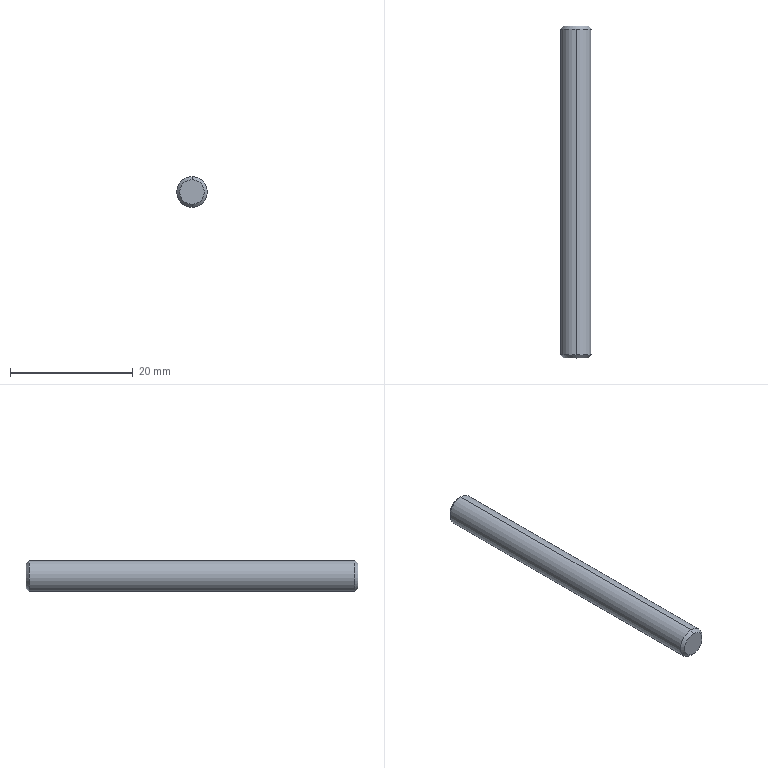Part | STEP file | SecondRearHHPMGS6pin_Default | 1 solid | 8 faces | box 5 x 54 x 5 mm | volume 1057 mm3 | cone 4 | cylinder 2 | plane 2 | commonest cylinder face diameters 5 x2
STEP:
#1=CARTESIAN_POINT('',(0.,0.,0.));
#2=DIRECTION('',(0.,0.,1.));
#3=DIRECTION('',(1.,0.,0.));
#4=AXIS2_PLACEMENT_3D('',#1,#2,#3);
#5=CARTESIAN_POINT('',(0.,-27.,2.));
#6=VERTEX_POINT('',#5);
#7=CARTESIAN_POINT('',(0.,-27.,-2.));
#8=VERTEX_POINT('',#7);
#9=CARTESIAN_POINT('',(0.,-27.,0.));
#10=DIRECTION('',(0.,1.,0.));
#11=DIRECTION('',(0.,0.,1.));
#12=AXIS2_PLACEMENT_3D('',#9,#10,#11);
#13=CIRCLE('',#12,2.);
#14=CARTESIAN_POINT('',(0.,-27.,0.));
#15=DIRECTION('',(0.,1.,0.));
#16=DIRECTION('',(0.,0.,1.));
#17=AXIS2_PLACEMENT_3D('',#14,#15,#16);
#18=CONICAL_SURFACE('',#17,2.,0.7854);
#19=CARTESIAN_POINT('',(0.,0.));
#20=DIRECTION('',(1.,0.));
#21=VECTOR('',#20,1.);
#22=LINE('',#19,#21);
#23=(GEOMETRIC_REPRESENTATION_CONTEXT(2)PARAMETRIC_REPRESENTATION_CONTEXT()REPRESENTATION_CONTEXT('',''));
#24=DEFINITIONAL_REPRESENTATION('',(#22),#23);
#25=PCURVE('',#18,#24);
#26=CARTESIAN_POINT('',(2.,-27.,0.));
#27=DIRECTION('',(0.,1.,0.));
#28=DIRECTION('',(0.,0.,1.));
#29=AXIS2_PLACEMENT_3D('',#26,#27,#28);
#30=PLANE('',#29);
#31=CARTESIAN_POINT('',(0.,-2.));
#32=DIRECTION('',(1.,0.));
#33=AXIS2_PLACEMENT_2D('',#31,#32);
#34=CIRCLE('',#33,2.);
#35=(GEOMETRIC_REPRESENTATION_CONTEXT(2)PARAMETRIC_REPRESENTATION_CONTEXT()REPRESENTATION_CONTEXT('',''));
#36=DEFINITIONAL_REPRESENTATION('',(#34),#35);
#37=PCURVE('',#30,#36);
#38=SURFACE_CURVE('',#13,(#25,#37),.PCURVE_S1.);
#39=EDGE_CURVE('',#6,#8,#38,.T.);
#40=ORIENTED_EDGE('',*,*,#39,.T.);
#41=CARTESIAN_POINT('',(0.,-26.5,-2.5));
#42=VERTEX_POINT('',#41);
#43=CARTESIAN_POINT('',(0.,-27.,-2.));
#44=DIRECTION('',(0.,0.7071,-0.7071));
#45=VECTOR('',#44,1.);
#46=LINE('',#43,#45);
#47=CARTESIAN_POINT('',(3.142,0.));
#48=DIRECTION('',(0.,1.));
#49=VECTOR('',#48,1.);
#50=LINE('',#47,#49);
#51=(GEOMETRIC_REPRESENTATION_CONTEXT(2)PARAMETRIC_REPRESENTATION_CONTEXT()REPRESENTATION_CONTEXT('',''));
#52=DEFINITIONAL_REPRESENTATION('',(#50),#51);
#53=PCURVE('',#18,#52);
#54=CARTESIAN_POINT('',(0.,-27.,0.));
#55=DIRECTION('',(0.,1.,0.));
#56=DIRECTION('',(0.,0.,1.));
#57=AXIS2_PLACEMENT_3D('',#54,#55,#56);
#58=CONICAL_SURFACE('',#57,2.,0.7854);
#59=CARTESIAN_POINT('',(3.142,0.));
#60=DIRECTION('',(0.,1.));
#61=VECTOR('',#60,1.);
#62=LINE('',#59,#61);
#63=(GEOMETRIC_REPRESENTATION_CONTEXT(2)PARAMETRIC_REPRESENTATION_CONTEXT()REPRESENTATION_CONTEXT('',''));
#64=DEFINITIONAL_REPRESENTATION('',(#62),#63);
#65=PCURVE('',#58,#64);
#66=SURFACE_CURVE('',#46,(#53,#65),.PCURVE_S1.);
#67=EDGE_CURVE('',#8,#42,#66,.T.);
#68=ORIENTED_EDGE('',*,*,#67,.T.);
#69=CARTESIAN_POINT('',(0.,-26.5,2.5));
#70=VERTEX_POINT('',#69);
#71=CARTESIAN_POINT('',(0.,-26.5,0.));
#72=DIRECTION('',(0.,1.,0.));
#73=DIRECTION('',(0.,0.,1.));
#74=AXIS2_PLACEMENT_3D('',#71,#72,#73);
#75=CIRCLE('',#74,2.5);
#76=CARTESIAN_POINT('',(0.,0.5));
#77=DIRECTION('',(1.,0.));
#78=VECTOR('',#77,1.);
#79=LINE('',#76,#78);
#80=(GEOMETRIC_REPRESENTATION_CONTEXT(2)PARAMETRIC_REPRESENTATION_CONTEXT()REPRESENTATION_CONTEXT('',''));
#81=DEFINITIONAL_REPRESENTATION('',(#79),#80);
#82=PCURVE('',#18,#81);
#83=CARTESIAN_POINT('',(0.,-27.,0.));
#84=DIRECTION('',(0.,1.,0.));
#85=DIRECTION('',(0.,0.,1.));
#86=AXIS2_PLACEMENT_3D('',#83,#84,#85);
#87=CYLINDRICAL_SURFACE('',#86,2.5);
#88=CARTESIAN_POINT('',(0.,0.5));
#89=DIRECTION('',(1.,0.));
#90=VECTOR('',#89,1.);
#91=LINE('',#88,#90);
#92=(GEOMETRIC_REPRESENTATION_CONTEXT(2)PARAMETRIC_REPRESENTATION_CONTEXT()REPRESENTATION_CONTEXT('',''));
#93=DEFINITIONAL_REPRESENTATION('',(#91),#92);
#94=PCURVE('',#87,#93);
#95=SURFACE_CURVE('',#75,(#82,#94),.PCURVE_S1.);
#96=EDGE_CURVE('',#70,#42,#95,.T.);
#97=ORIENTED_EDGE('',*,*,#96,.F.);
#98=CARTESIAN_POINT('',(0.,-27.,2.));
#99=DIRECTION('',(0.,0.7071,0.7071));
#100=VECTOR('',#99,1.);
#101=LINE('',#98,#100);
#102=CARTESIAN_POINT('',(0.,0.));
#103=DIRECTION('',(0.,1.));
#104=VECTOR('',#103,1.);
#105=LINE('',#102,#104);
#106=(GEOMETRIC_REPRESENTATION_CONTEXT(2)PARAMETRIC_REPRESENTATION_CONTEXT()REPRESENTATION_CONTEXT('',''));
#107=DEFINITIONAL_REPRESENTATION('',(#105),#106);
#108=PCURVE('',#18,#107);
#109=CARTESIAN_POINT('',(6.283,0.));
#110=DIRECTION('',(0.,1.));
#111=VECTOR('',#110,1.);
#112=LINE('',#109,#111);
#113=(GEOMETRIC_REPRESENTATION_CONTEXT(2)PARAMETRIC_REPRESENTATION_CONTEXT()REPRESENTATION_CONTEXT('',''));
#114=DEFINITIONAL_REPRESENTATION('',(#112),#113);
#115=PCURVE('',#58,#114);
#116=SURFACE_CURVE('',#101,(#108,#115),.PCURVE_S1.);
#117=EDGE_CURVE('',#6,#70,#116,.T.);
#118=ORIENTED_EDGE('',*,*,#117,.F.);
#119=EDGE_LOOP('',(#40,#68,#97,#118));
#120=FACE_BOUND('',#119,.T.);
#121=ADVANCED_FACE('',(#120),#18,.T.);
#122=ORIENTED_EDGE('',*,*,#96,.T.);
#123=CARTESIAN_POINT('',(0.,26.5,-2.5));
#124=VERTEX_POINT('',#123);
#125=CARTESIAN_POINT('',(0.,-27.,-2.5));
#126=DIRECTION('',(0.,1.,0.));
#127=VECTOR('',#126,1.);
#128=LINE('',#125,#127);
#129=CARTESIAN_POINT('',(3.142,0.));
#130=DIRECTION('',(0.,1.));
#131=VECTOR('',#130,1.);
#132=LINE('',#129,#131);
#133=(GEOMETRIC_REPRESENTATION_CONTEXT(2)PARAMETRIC_REPRESENTATION_CONTEXT()REPRESENTATION_CONTEXT('',''));
#134=DEFINITIONAL_REPRESENTATION('',(#132),#133);
#135=PCURVE('',#87,#134);
#136=CARTESIAN_POINT('',(0.,-27.,0.));
#137=DIRECTION('',(0.,1.,0.));
#138=DIRECTION('',(0.,0.,1.));
#139=AXIS2_PLACEMENT_3D('',#136,#137,#138);
#140=CYLINDRICAL_SURFACE('',#139,2.5);
#141=CARTESIAN_POINT('',(3.142,0.));
#142=DIRECTION('',(0.,1.));
#143=VECTOR('',#142,1.);
#144=LINE('',#141,#143);
#145=(GEOMETRIC_REPRESENTATION_CONTEXT(2)PARAMETRIC_REPRESENTATION_CONTEXT()REPRESENTATION_CONTEXT('',''));
#146=DEFINITIONAL_REPRESENTATION('',(#144),#145);
#147=PCURVE('',#140,#146);
#148=SURFACE_CURVE('',#128,(#135,#147),.PCURVE_S1.);
#149=EDGE_CURVE('',#42,#124,#148,.T.);
#150=ORIENTED_EDGE('',*,*,#149,.T.);
#151=CARTESIAN_POINT('',(0.,26.5,2.5));
#152=VERTEX_POINT('',#151);
#153=CARTESIAN_POINT('',(0.,26.5,0.));
#154=DIRECTION('',(0.,1.,0.));
#155=DIRECTION('',(0.,0.,1.));
#156=AXIS2_PLACEMENT_3D('',#153,#154,#155);
#157=CIRCLE('',#156,2.5);
#158=CARTESIAN_POINT('',(0.,53.5));
#159=DIRECTION('',(1.,0.));
#160=VECTOR('',#159,1.);
#161=LINE('',#158,#160);
#162=(GEOMETRIC_REPRESENTATION_CONTEXT(2)PARAMETRIC_REPRESENTATION_CONTEXT()REPRESENTATION_CONTEXT('',''));
#163=DEFINITIONAL_REPRESENTATION('',(#161),#162);
#164=PCURVE('',#87,#163);
#165=CARTESIAN_POINT('',(0.,26.5,0.));
#166=DIRECTION('',(0.,-1.,0.));
#167=DIRECTION('',(0.,0.,-1.));
#168=AXIS2_PLACEMENT_3D('',#165,#166,#167);
#169=CONICAL_SURFACE('',#168,2.5,0.7854);
#170=CARTESIAN_POINT('',(3.142,0.));
#171=DIRECTION('',(-1.,0.));
#172=VECTOR('',#171,1.);
#173=LINE('',#170,#172);
#174=(GEOMETRIC_REPRESENTATION_CONTEXT(2)PARAMETRIC_REPRESENTATION_CONTEXT()REPRESENTATION_CONTEXT('',''));
#175=DEFINITIONAL_REPRESENTATION('',(#173),#174);
#176=PCURVE('',#169,#175);
#177=SURFACE_CURVE('',#157,(#164,#176),.PCURVE_S1.);
#178=EDGE_CURVE('',#152,#124,#177,.T.);
#179=ORIENTED_EDGE('',*,*,#178,.F.);
#180=CARTESIAN_POINT('',(0.,-27.,2.5));
#181=DIRECTION('',(0.,1.,0.));
#182=VECTOR('',#181,1.);
#183=LINE('',#180,#182);
#184=CARTESIAN_POINT('',(0.,0.));
#185=DIRECTION('',(0.,1.));
#186=VECTOR('',#185,1.);
#187=LINE('',#184,#186);
#188=(GEOMETRIC_REPRESENTATION_CONTEXT(2)PARAMETRIC_REPRESENTATION_CONTEXT()REPRESENTATION_CONTEXT('',''));
#189=DEFINITIONAL_REPRESENTATION('',(#187),#188);
#190=PCURVE('',#87,#189);
#191=CARTESIAN_POINT('',(6.283,0.));
#192=DIRECTION('',(0.,1.));
#193=VECTOR('',#192,1.);
#194=LINE('',#191,#193);
#195=(GEOMETRIC_REPRESENTATION_CONTEXT(2)PARAMETRIC_REPRESENTATION_CONTEXT()REPRESENTATION_CONTEXT('',''));
#196=DEFINITIONAL_REPRESENTATION('',(#194),#195);
#197=PCURVE('',#140,#196);
#198=SURFACE_CURVE('',#183,(#190,#197),.PCURVE_S1.);
#199=EDGE_CURVE('',#70,#152,#198,.T.);
#200=ORIENTED_EDGE('',*,*,#199,.F.);
#201=EDGE_LOOP('',(#122,#150,#179,#200));
#202=FACE_BOUND('',#201,.T.);
#203=ADVANCED_FACE('',(#202),#87,.T.);
#204=CARTESIAN_POINT('',(0.,27.,2.));
#205=VERTEX_POINT('',#204);
#206=CARTESIAN_POINT('',(0.,27.,-2.));
#207=VERTEX_POINT('',#206);
#208=CARTESIAN_POINT('',(0.,27.,0.));
#209=DIRECTION('',(0.,1.,0.));
#210=DIRECTION('',(0.,0.,1.));
#211=AXIS2_PLACEMENT_3D('',#208,#209,#210);
#212=CIRCLE('',#211,2.);
#213=CARTESIAN_POINT('',(3.142,-0.5));
#214=DIRECTION('',(-1.,0.));
#215=VECTOR('',#214,1.);
#216=LINE('',#213,#215);
#217=(GEOMETRIC_REPRESENTATION_CONTEXT(2)PARAMETRIC_REPRESENTATION_CONTEXT()REPRESENTATION_CONTEXT('',''));
#218=DEFINITIONAL_REPRESENTATION('',(#216),#217);
#219=PCURVE('',#169,#218);
#220=CARTESIAN_POINT('',(0.,27.,0.));
#221=DIRECTION('',(0.,-1.,0.));
#222=DIRECTION('',(0.,0.,-1.));
#223=AXIS2_PLACEMENT_3D('',#220,#221,#222);
#224=PLANE('',#223);
#225=CARTESIAN_POINT('',(-2.,0.));
#226=CARTESIAN_POINT('',(-2.,3.464));
#227=CARTESIAN_POINT('',(1.,1.732));
#228=CARTESIAN_POINT('',(4.,0.));
#229=CARTESIAN_POINT('',(1.,-1.732));
#230=CARTESIAN_POINT('',(-2.,-3.464));
#231=CARTESIAN_POINT('',(-2.,0.));
#232=(BOUNDED_CURVE()B_SPLINE_CURVE(2,(#225,#226,#227,#228,#229,#230,#231),.UNSPECIFIED.,.T.,.F.)B_SPLINE_CURVE_WITH_KNOTS((1,2,2,2,2,1),(-2.094,0.,2.094,4.189,6.283,8.378),.UNSPECIFIED.)CURVE()GEOMETRIC_REPRESENTATION_ITEM()RATIONAL_B_SPLINE_CURVE((1.,0.5,1.,0.5,1.,0.5,1.))REPRESENTATION_ITEM(''));
#233=(GEOMETRIC_REPRESENTATION_CONTEXT(2)PARAMETRIC_REPRESENTATION_CONTEXT()REPRESENTATION_CONTEXT('',''));
#234=DEFINITIONAL_REPRESENTATION('',(#232),#233);
#235=PCURVE('',#224,#234);
#236=SURFACE_CURVE('',#212,(#219,#235),.PCURVE_S1.);
#237=EDGE_CURVE('',#205,#207,#236,.T.);
#238=ORIENTED_EDGE('',*,*,#237,.F.);
#239=CARTESIAN_POINT('',(0.,26.5,2.5));
#240=DIRECTION('',(0.,-0.7071,0.7071));
#241=VECTOR('',#240,1.);
#242=LINE('',#239,#241);
#243=CARTESIAN_POINT('',(3.142,0.));
#244=DIRECTION('',(0.,1.));
#245=VECTOR('',#244,1.);
#246=LINE('',#243,#245);
#247=(GEOMETRIC_REPRESENTATION_CONTEXT(2)PARAMETRIC_REPRESENTATION_CONTEXT()REPRESENTATION_CONTEXT('',''));
#248=DEFINITIONAL_REPRESENTATION('',(#246),#247);
#249=PCURVE('',#169,#248);
#250=CARTESIAN_POINT('',(0.,26.5,0.));
#251=DIRECTION('',(0.,-1.,0.));
#252=DIRECTION('',(0.,0.,-1.));
#253=AXIS2_PLACEMENT_3D('',#250,#251,#252);
#254=CONICAL_SURFACE('',#253,2.5,0.7854);
#255=CARTESIAN_POINT('',(3.142,0.));
#256=DIRECTION('',(0.,1.));
#257=VECTOR('',#256,1.);
#258=LINE('',#255,#257);
#259=(GEOMETRIC_REPRESENTATION_CONTEXT(2)PARAMETRIC_REPRESENTATION_CONTEXT()REPRESENTATION_CONTEXT('',''));
#260=DEFINITIONAL_REPRESENTATION('',(#258),#259);
#261=PCURVE('',#254,#260);
#262=SURFACE_CURVE('',#242,(#249,#261),.PCURVE_S1.);
#263=EDGE_CURVE('',#205,#152,#262,.T.);
#264=ORIENTED_EDGE('',*,*,#263,.T.);
#265=ORIENTED_EDGE('',*,*,#178,.T.);
#266=CARTESIAN_POINT('',(0.,26.5,-2.5));
#267=DIRECTION('',(0.,-0.7071,-0.7071));
#268=VECTOR('',#267,1.);
#269=LINE('',#266,#268);
#270=CARTESIAN_POINT('',(0.,0.));
#271=DIRECTION('',(0.,1.));
#272=VECTOR('',#271,1.);
#273=LINE('',#270,#272);
#274=(GEOMETRIC_REPRESENTATION_CONTEXT(2)PARAMETRIC_REPRESENTATION_CONTEXT()REPRESENTATION_CONTEXT('',''));
#275=DEFINITIONAL_REPRESENTATION('',(#273),#274);
#276=PCURVE('',#169,#275);
#277=CARTESIAN_POINT('',(6.283,0.));
#278=DIRECTION('',(0.,1.));
#279=VECTOR('',#278,1.);
#280=LINE('',#277,#279);
#281=(GEOMETRIC_REPRESENTATION_CONTEXT(2)PARAMETRIC_REPRESENTATION_CONTEXT()REPRESENTATION_CONTEXT('',''));
#282=DEFINITIONAL_REPRESENTATION('',(#280),#281);
#283=PCURVE('',#254,#282);
#284=SURFACE_CURVE('',#269,(#276,#283),.PCURVE_S1.);
#285=EDGE_CURVE('',#207,#124,#284,.T.);
#286=ORIENTED_EDGE('',*,*,#285,.F.);
#287=EDGE_LOOP('',(#238,#264,#265,#286));
#288=FACE_BOUND('',#287,.T.);
#289=ADVANCED_FACE('',(#288),#169,.T.);
#290=CARTESIAN_POINT('',(0.,27.,0.));
#291=DIRECTION('',(0.,1.,0.));
#292=DIRECTION('',(0.,0.,1.));
#293=AXIS2_PLACEMENT_3D('',#290,#291,#292);
#294=CIRCLE('',#293,2.);
#295=CARTESIAN_POINT('',(-2.,0.));
#296=CARTESIAN_POINT('',(-2.,3.464));
#297=CARTESIAN_POINT('',(1.,1.732));
#298=CARTESIAN_POINT('',(4.,0.));
#299=CARTESIAN_POINT('',(1.,-1.732));
#300=CARTESIAN_POINT('',(-2.,-3.464));
#301=CARTESIAN_POINT('',(-2.,0.));
#302=(BOUNDED_CURVE()B_SPLINE_CURVE(2,(#295,#296,#297,#298,#299,#300,#301),.UNSPECIFIED.,.T.,.F.)B_SPLINE_CURVE_WITH_KNOTS((1,2,2,2,2,1),(-2.094,0.,2.094,4.189,6.283,8.378),.UNSPECIFIED.)CURVE()GEOMETRIC_REPRESENTATION_ITEM()RATIONAL_B_SPLINE_CURVE((1.,0.5,1.,0.5,1.,0.5,1.))REPRESENTATION_ITEM(''));
#303=(GEOMETRIC_REPRESENTATION_CONTEXT(2)PARAMETRIC_REPRESENTATION_CONTEXT()REPRESENTATION_CONTEXT('',''));
#304=DEFINITIONAL_REPRESENTATION('',(#302),#303);
#305=PCURVE('',#224,#304);
#306=CARTESIAN_POINT('',(9.425,-0.5));
#307=DIRECTION('',(-1.,0.));
#308=VECTOR('',#307,1.);
#309=LINE('',#306,#308);
#310=(GEOMETRIC_REPRESENTATION_CONTEXT(2)PARAMETRIC_REPRESENTATION_CONTEXT()REPRESENTATION_CONTEXT('',''));
#311=DEFINITIONAL_REPRESENTATION('',(#309),#310);
#312=PCURVE('',#254,#311);
#313=SURFACE_CURVE('',#294,(#305,#312),.PCURVE_S1.);
#314=EDGE_CURVE('',#207,#205,#313,.T.);
#315=ORIENTED_EDGE('',*,*,#314,.T.);
#316=ORIENTED_EDGE('',*,*,#237,.T.);
#317=EDGE_LOOP('',(#315,#316));
#318=FACE_BOUND('',#317,.T.);
#319=ADVANCED_FACE('',(#318),#224,.F.);
#320=ORIENTED_EDGE('',*,*,#263,.F.);
#321=ORIENTED_EDGE('',*,*,#314,.F.);
#322=ORIENTED_EDGE('',*,*,#285,.T.);
#323=CARTESIAN_POINT('',(0.,26.5,0.));
#324=DIRECTION('',(0.,1.,0.));
#325=DIRECTION('',(0.,0.,1.));
#326=AXIS2_PLACEMENT_3D('',#323,#324,#325);
#327=CIRCLE('',#326,2.5);
#328=CARTESIAN_POINT('',(9.425,0.));
#329=DIRECTION('',(-1.,0.));
#330=VECTOR('',#329,1.);
#331=LINE('',#328,#330);
#332=(GEOMETRIC_REPRESENTATION_CONTEXT(2)PARAMETRIC_REPRESENTATION_CONTEXT()REPRESENTATION_CONTEXT('',''));
#333=DEFINITIONAL_REPRESENTATION('',(#331),#332);
#334=PCURVE('',#254,#333);
#335=CARTESIAN_POINT('',(0.,53.5));
#336=DIRECTION('',(1.,0.));
#337=VECTOR('',#336,1.);
#338=LINE('',#335,#337);
#339=(GEOMETRIC_REPRESENTATION_CONTEXT(2)PARAMETRIC_REPRESENTATION_CONTEXT()REPRESENTATION_CONTEXT('',''));
#340=DEFINITIONAL_REPRESENTATION('',(#338),#339);
#341=PCURVE('',#140,#340);
#342=SURFACE_CURVE('',#327,(#334,#341),.PCURVE_S1.);
#343=EDGE_CURVE('',#124,#152,#342,.T.);
#344=ORIENTED_EDGE('',*,*,#343,.T.);
#345=EDGE_LOOP('',(#320,#321,#322,#344));
#346=FACE_BOUND('',#345,.T.);
#347=ADVANCED_FACE('',(#346),#254,.T.);
#348=ORIENTED_EDGE('',*,*,#149,.F.);
#349=CARTESIAN_POINT('',(0.,-26.5,0.));
#350=DIRECTION('',(0.,1.,0.));
#351=DIRECTION('',(0.,0.,1.));
#352=AXIS2_PLACEMENT_3D('',#349,#350,#351);
#353=CIRCLE('',#352,2.5);
#354=CARTESIAN_POINT('',(0.,0.5));
#355=DIRECTION('',(1.,0.));
#356=VECTOR('',#355,1.);
#357=LINE('',#354,#356);
#358=(GEOMETRIC_REPRESENTATION_CONTEXT(2)PARAMETRIC_REPRESENTATION_CONTEXT()REPRESENTATION_CONTEXT('',''));
#359=DEFINITIONAL_REPRESENTATION('',(#357),#358);
#360=PCURVE('',#140,#359);
#361=CARTESIAN_POINT('',(0.,0.5));
#362=DIRECTION('',(1.,0.));
#363=VECTOR('',#362,1.);
#364=LINE('',#361,#363);
#365=(GEOMETRIC_REPRESENTATION_CONTEXT(2)PARAMETRIC_REPRESENTATION_CONTEXT()REPRESENTATION_CONTEXT('',''));
#366=DEFINITIONAL_REPRESENTATION('',(#364),#365);
#367=PCURVE('',#58,#366);
#368=SURFACE_CURVE('',#353,(#360,#367),.PCURVE_S1.);
#369=EDGE_CURVE('',#42,#70,#368,.T.);
#370=ORIENTED_EDGE('',*,*,#369,.T.);
#371=ORIENTED_EDGE('',*,*,#199,.T.);
#372=ORIENTED_EDGE('',*,*,#343,.F.);
#373=EDGE_LOOP('',(#348,#370,#371,#372));
#374=FACE_BOUND('',#373,.T.);
#375=ADVANCED_FACE('',(#374),#140,.T.);
#376=ORIENTED_EDGE('',*,*,#67,.F.);
#377=CARTESIAN_POINT('',(0.,-27.,0.));
#378=DIRECTION('',(0.,1.,0.));
#379=DIRECTION('',(0.,0.,1.));
#380=AXIS2_PLACEMENT_3D('',#377,#378,#379);
#381=CIRCLE('',#380,2.);
#382=CARTESIAN_POINT('',(0.,0.));
#383=DIRECTION('',(1.,0.));
#384=VECTOR('',#383,1.);
#385=LINE('',#382,#384);
#386=(GEOMETRIC_REPRESENTATION_CONTEXT(2)PARAMETRIC_REPRESENTATION_CONTEXT()REPRESENTATION_CONTEXT('',''));
#387=DEFINITIONAL_REPRESENTATION('',(#385),#386);
#388=PCURVE('',#58,#387);
#389=CARTESIAN_POINT('',(0.,-2.));
#390=DIRECTION('',(1.,0.));
#391=AXIS2_PLACEMENT_2D('',#389,#390);
#392=CIRCLE('',#391,2.);
#393=(GEOMETRIC_REPRESENTATION_CONTEXT(2)PARAMETRIC_REPRESENTATION_CONTEXT()REPRESENTATION_CONTEXT('',''));
#394=DEFINITIONAL_REPRESENTATION('',(#392),#393);
#395=PCURVE('',#30,#394);
#396=SURFACE_CURVE('',#381,(#388,#395),.PCURVE_S1.);
#397=EDGE_CURVE('',#8,#6,#396,.T.);
#398=ORIENTED_EDGE('',*,*,#397,.T.);
#399=ORIENTED_EDGE('',*,*,#117,.T.);
#400=ORIENTED_EDGE('',*,*,#369,.F.);
#401=EDGE_LOOP('',(#376,#398,#399,#400));
#402=FACE_BOUND('',#401,.T.);
#403=ADVANCED_FACE('',(#402),#58,.T.);
#404=ORIENTED_EDGE('',*,*,#39,.F.);
#405=ORIENTED_EDGE('',*,*,#397,.F.);
#406=EDGE_LOOP('',(#404,#405));
#407=FACE_BOUND('',#406,.T.);
#408=ADVANCED_FACE('',(#407),#30,.F.);
#409=CLOSED_SHELL('',(#121,#203,#289,#319,#347,#375,#403,#408));
#410=MANIFOLD_SOLID_BREP('',#409);
#411=(LENGTH_UNIT()NAMED_UNIT(*)SI_UNIT(.MILLI.,.METRE.));
#412=UNCERTAINTY_MEASURE_WITH_UNIT(LENGTH_MEASURE(0.0000001),#411,'','');
#413=(NAMED_UNIT(*)PLANE_ANGLE_UNIT()SI_UNIT($,.RADIAN.));
#414=(NAMED_UNIT(*)SI_UNIT($,.STERADIAN.)SOLID_ANGLE_UNIT());
#415=(GEOMETRIC_REPRESENTATION_CONTEXT(3)GLOBAL_UNCERTAINTY_ASSIGNED_CONTEXT((#412))GLOBAL_UNIT_ASSIGNED_CONTEXT((#411,#413,#414))REPRESENTATION_CONTEXT('',''));
#416=ADVANCED_BREP_SHAPE_REPRESENTATION('',(#4,#410),#415);